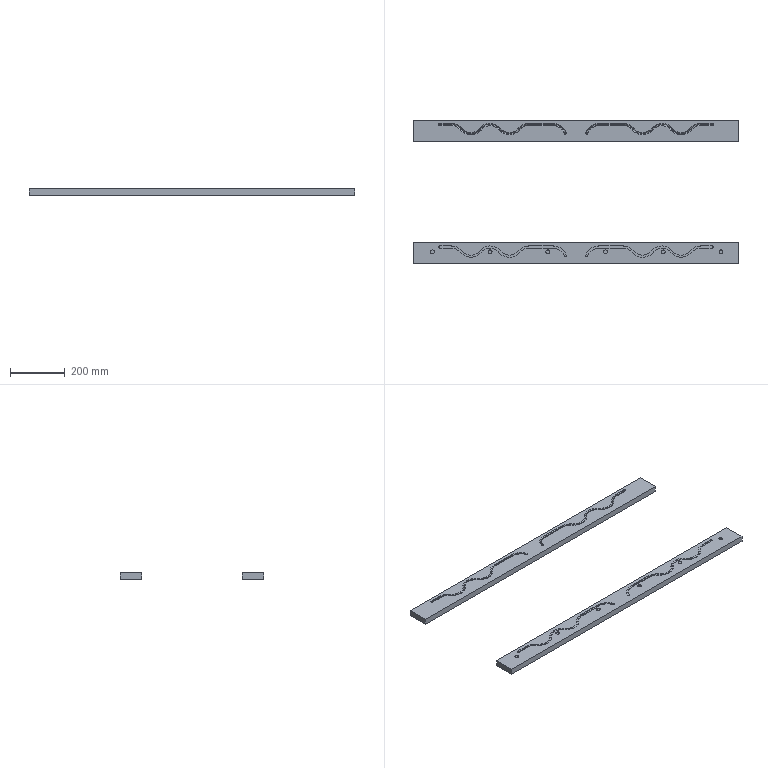NC program | NX | posted with a generic post | part box 1185 x 523.484 x 22 mm
Lines 1046 to 2009 of 261559:
(定轴曲面加工 , TOOL : D3平底刀)
N2072 T15 M6
N2074 /M1
N2076 G54
N2078 G17 G0 G90 X22.96 Y24.701 S3000 M3
N2080 G43 Z50. H15
N2082 Z1.5
N2084 G94 G1 X23.024 Y24.738 Z1.036 F2450.
N2086 X23.208 Y24.845 Z0.618
N2088 X23.495 Y25.012 Z0.286
N2090 X23.856 Y25.223 Z0.073
N2092 X24.257 Y25.456 Z0.
N2094 X24.643 Y25.681 F3500.
N2096 X25.42 Y26.134
N2098 X25.799 Y26.355
N2100 X25.809 Y26.359
N2102 X26.024 Y26.417
N2104 X26.049 Y26.42
N2106 X26.06 Y26.394
N2108 X26.039 Y26.379
N2110 X25.471 Y26.048
N2112 X24.693 Y25.595
N2114 X24. Y25.191
N2116 X23.995 Y25.187
N2118 X23.982 Y25.174
N2120 X23.826 Y24.987
N2122 X23.822 Y24.983
N2124 X23.826 Y24.98
N2126 X23.83 Y24.975
N2128 X23.834 Y24.979
N2130 X23.966 Y25.055
N2132 X24.743 Y25.508
N2134 X25.521 Y25.961
N2136 X26.299 Y26.414
N2138 X26.446 Y26.5
N2140 X26.464 Y26.506
N2142 X26.537 Y26.515
N2144 X26.573 Y26.512
N2146 X26.585 Y26.474
N2148 X26.558 Y26.45
N2150 X26.349 Y26.328
N2152 X25.571 Y25.875
N2154 X24.794 Y25.422
N2156 X24.016 Y24.969
N2158 X23.673 Y24.769
N2160 X23.666 Y24.762
N2162 X23.65 Y24.743
N2164 X23.571 Y24.621
N2166 X23.563 Y24.612
N2168 X23.572 Y24.605
N2170 X23.579 Y24.596
N2172 X23.587 Y24.603
N2174 X24.066 Y24.882
N2176 X24.844 Y25.335
N2178 X25.622 Y25.789
N2180 X26.399 Y26.242
N2182 X26.906 Y26.537
N2184 X26.929 Y26.544
N2186 X26.975 Y26.546
N2188 X27.013 Y26.54
N2190 X27.025 Y26.5
N2192 X26.997 Y26.474
N2194 X26.45 Y26.155
N2196 X25.672 Y25.702
N2198 X24.894 Y25.249
N2200 X24.117 Y24.796
N2202 X23.459 Y24.413
N2204 X23.45 Y24.404
N2206 X23.433 Y24.38
N2208 X23.391 Y24.298
N2210 X23.38 Y24.285
N2212 X23.395 Y24.276
N2214 X23.405 Y24.261
N2216 X23.418 Y24.273
N2218 X24.167 Y24.71
N2220 X24.945 Y25.163
N2222 X25.722 Y25.616
N2224 X26.5 Y26.069
N2226 X27.278 Y26.522
N2228 X27.328 Y26.551
N2230 X27.353 Y26.558
N2232 X27.395
N2234 X27.432 Y26.551
N2236 X27.443 Y26.512
N2238 X27.415 Y26.486
N2240 X27.328 Y26.436
N2242 X26.55 Y25.983
N2244 X25.773 Y25.529
N2246 X24.995 Y25.076
N2248 X24.217 Y24.623
N2250 X23.44 Y24.17
N2252 X23.306 Y24.092
N2254 X23.296 Y24.081
N2256 X23.279 Y24.053
N2258 X23.251 Y23.985
N2260 X23.241 Y23.971
N2262 X23.256 Y23.964
N2264 X23.267 Y23.949
N2266 X23.28 Y23.961
N2268 X23.49 Y24.084
N2270 X24.268 Y24.537
N2272 X25.045 Y24.99
N2274 X25.823 Y25.443
N2276 X26.601 Y25.896
N2278 X27.378 Y26.349
N2280 X27.73 Y26.554
N2282 X27.755 Y26.561
N2284 X27.797 Y26.562
N2286 X27.835 Y26.554
N2288 X27.846 Y26.515
N2290 X27.817 Y26.489
N2292 X27.429 Y26.263
N2294 X26.651 Y25.81
N2296 X25.873 Y25.357
N2298 X25.096 Y24.904
N2300 X24.318 Y24.45
N2302 X23.54 Y23.997
N2304 X23.194 Y23.796
N2306 X23.184 Y23.783
N2308 X23.166 Y23.75
N2310 X23.148 Y23.693
N2312 X23.139 Y23.679
N2314 X23.154 Y23.673
N2316 X23.155 Y23.672
N2318 X23.165 Y23.658
N2320 X23.178 Y23.67
N2322 X23.591 Y23.911
N2324 X24.368 Y24.364
N2326 X25.146 Y24.817
N2328 X25.924 Y25.27
N2330 X26.701 Y25.723
N2332 X27.479 Y26.177
N2334 X28.133 Y26.558
N2336 X28.157 Y26.564
N2338 X28.2 Y26.565
N2340 X28.237 Y26.557
N2342 X28.248 Y26.518
N2344 X28.22 Y26.492
N2346 X27.529 Y26.09
N2348 X26.752 Y25.637
N2350 X25.974 Y25.184
N2352 X25.196 Y24.731
N2354 X24.419 Y24.278
N2356 X23.641 Y23.825
N2358 X23.112 Y23.516
N2360 X23.101 Y23.502
N2362 X23.084 Y23.466
N2364 X23.076 Y23.433
N2366 X23.067 Y23.415
N2368 X23.086 Y23.406
N2370 X23.087
N2372 X23.101 Y23.39
N2374 X23.118 Y23.404
N2376 X23.691 Y23.738
N2378 X24.469 Y24.191
N2380 X25.247 Y24.644
N2382 X26.024 Y25.098
N2384 X26.802 Y25.551
N2386 X27.58 Y26.004
N2388 X28.357 Y26.457
N2390 X28.535 Y26.561
N2392 X28.56 Y26.567
N2394 X28.602 Y26.568
N2396 X28.639 Y26.56
N2398 X28.65 Y26.521
N2400 X28.622 Y26.495
N2402 X28.408 Y26.37
N2404 X27.63 Y25.917
N2406 X26.852 Y25.464
N2408 X26.075 Y25.011 Z-0.001
N2410 X25.297 Y24.558 Z-0.002
N2412 X24.519 Y24.105 Z0.
N2414 X23.742 Y23.652
N2416 X23.054 Y23.251
N2418 X23.043 Y23.235
N2420 X23.023 Y23.22
N2422 X23.027 Y23.195
N2424 X23.022 Y23.171
N2426 X23.015 Y23.151
N2428 X23.034 Y23.143
N2430 X23.049 Y23.128
N2432 X23.064 Y23.141
N2434 X23.792 Y23.565
N2436 X24.57 Y24.019
N2438 X25.347 Y24.472 Z-0.011
N2440 X26.125 Y24.925
N2442 X26.903 Y25.378 Z0.
N2444 X27.68 Y25.831
N2446 X28.458 Y26.284
N2448 X28.934 Y26.561
N2450 X28.959 Y26.568
N2452 X29.
N2454 X29.038 Y26.561
N2456 X29.048 Y26.521
N2458 X29.02 Y26.496
N2460 X28.508 Y26.198
N2462 X27.731 Y25.745
N2464 X26.953 Y25.292
N2466 X26.175 Y24.838 Z-0.02
N2468 X25.398 Y24.385 Z-0.021
N2470 X24.62 Y23.932 Z0.
N2472 X23.842 Y23.479
N2474 X23.065 Y23.026
N2476 X23.016 Y22.998
N2478 X23.005 Y22.98
N2480 X22.985 Y22.963
N2482 X22.989 Y22.937
N2484 Y22.932
N2486 X22.983 Y22.909
N2488 X23.004 Y22.899
N2490 X23.006 Y22.898
N2492 X23.024 Y22.882
N2494 X23.042 Y22.897
N2496 X23.115 Y22.94
N2498 X23.893 Y23.393
N2500 X24.67 Y23.846
N2502 X25.448 Y24.299 Z-0.031
N2504 X26.226 Y24.752 Z-0.03
N2506 X27.003 Y25.205 Z0.
N2508 X27.781 Y25.658
N2510 X28.559 Y26.111
N2512 X29.331 Y26.562
N2514 X29.356 Y26.568
N2516 X29.398
N2518 X29.435 Y26.561
N2520 X29.446 Y26.521
N2522 X29.417 Y26.496
N2524 X29.386 Y26.478
N2526 X28.609 Y26.025
N2528 X27.831 Y25.572
N2530 X27.054 Y25.119 Z-0.005
N2532 X26.276 Y24.666 Z-0.04
N2534 X25.498 Y24.213
N2536 X24.721 Y23.759 Z-0.008
N2538 X23.943 Y23.306 Z0.
N2540 X23.166 Y22.853
N2542 X23.015 Y22.765
N2544 X22.99 Y22.759
N2546 X22.983 Y22.735
N2548 X22.982 Y22.733
N2550 X22.963 Y22.716
N2552 X22.969 Y22.691
N2554 Y22.688
N2556 X22.964 Y22.665
N2558 X22.986 Y22.656
N2560 X23.005 Y22.641
N2562 X23.025 Y22.656
N2564 X23.216 Y22.767
N2566 X23.993 Y23.22
N2568 X24.771 Y23.673 Z-0.017
N2570 X25.549 Y24.126 Z-0.068
N2572 X26.326 Y24.579 Z-0.066
N2574 X27.104 Y25.032 Z-0.011
N2576 X27.882 Y25.485 Z0.
N2578 X28.659 Y25.939
N2580 X29.437 Y26.392
N2582 X29.728 Y26.562
N2584 X29.754 Y26.568
N2586 X29.795
N2588 X29.833 Y26.561
N2590 X29.843 Y26.521
N2592 X29.815 Y26.496
N2594 X29.487 Y26.305
N2596 X28.71 Y25.852
N2598 X27.932 Y25.399
N2600 X27.154 Y24.946 Z-0.016
N2602 X26.377 Y24.493 Z-0.096
N2604 X25.599 Y24.04 Z-0.097
N2606 X24.821 Y23.587 Z-0.025
N2608 X24.044 Y23.134 Z0.
N2610 X23.266 Y22.68
N2612 X23.009 Y22.531
N2614 X22.984 Y22.524
N2616 X22.977 Y22.498
N2618 X22.974 Y22.493
N2620 X22.957 Y22.477
N2622 X22.964 Y22.456
N2624 Y22.452
N2626 X22.96 Y22.43
N2628 X22.982 Y22.422
N2630 X23.002 Y22.407
N2632 X23.021 Y22.422
N2634 X23.317 Y22.594
N2636 X24.094 Y23.047
N2638 X24.872 Y23.5 Z-0.033
N2640 X25.645 Y23.951 Z-0.127
N2642 X25.649 Y23.953
N2644 X25.654 Y23.956
N2646 X26.422 Y24.404 Z-0.126
N2648 X26.427 Y24.407
N2650 X26.432 Y24.409 Z-0.125
N2652 X27.205 Y24.86 Z-0.028
N2654 X27.982 Y25.313 Z0.
N2656 X28.76 Y25.766
N2658 X29.537 Y26.219
N2660 X30.126 Y26.562
N2662 X30.151 Y26.569
N2664 X30.193
N2666 X30.23 Y26.561
N2668 X30.241 Y26.522
N2670 X30.212 Y26.496
N2672 X29.588 Y26.133
N2674 X28.81 Y25.679
N2676 X28.033 Y25.226
N2678 X27.255 Y24.773 Z-0.042
N2680 X26.477 Y24.32 Z-0.155
N2682 X26.092 Y24.096 Z-0.176
N2684 X26.089 Y24.094
N2686 X26.085 Y24.091
N2688 X25.7 Y23.867 Z-0.157
N2690 X24.922 Y23.414 Z-0.042
N2692 X24.144 Y22.961 Z0.
N2694 X23.367 Y22.508
N2696 X23.018 Y22.304
N2698 X22.991 Y22.296
N2700 X22.984 Y22.269
N2702 X22.978 Y22.259
N2704 X22.972 Y22.23
N2706 Y22.228
N2708 X22.968 Y22.209
N2710 X22.987 Y22.205
N2712 X22.989 Y22.204
N2714 X23.018 Y22.187
N2716 X23.046 Y22.205
N2718 X23.417 Y22.421
N2720 X24.195 Y22.874
N2722 X24.972 Y23.328 Z-0.065
N2724 X25.746 Y23.778 Z-0.201
N2726 X25.75 Y23.781 Z-0.202
N2728 X25.754 Y23.783
N2730 X26.133 Y24.004 Z-0.229
N2732 X26.139 Y24.007 Z-0.23
N2734 X26.145 Y24.011 Z-0.229
N2736 X26.528 Y24.234 Z-0.197
N2738 X27.305 Y24.687 Z-0.062
N2740 X28.083 Y25.14 Z-0.004
N2742 X28.861 Y25.593 Z0.
N2744 X29.638 Y26.046
N2746 X30.416 Y26.499
N2748 X30.523 Y26.562
N2750 X30.548 Y26.569
N2752 X30.59
N2754 X30.627 Y26.561
N2756 X30.638 Y26.522
N2758 X30.61 Y26.497
N2760 X30.466 Y26.413
N2762 X29.688 Y25.96
N2764 X28.911 Y25.507
N2766 X28.133 Y25.054 Z-0.009
N2768 X27.356 Y24.6 Z-0.085
N2770 X26.582 Y24.15 Z-0.248
N2772 X26.578 Y24.147
N2774 X26.574 Y24.145 Z-0.249
N2776 X26.195 Y23.924 Z-0.283
N2778 X26.189 Y23.921
N2780 X26.183 Y23.917
N2782 X25.805 Y23.697 Z-0.254
N2784 X25.8 Y23.694
N2786 X25.795 Y23.691 Z-0.253
N2788 X25.023 Y23.241 Z-0.088
N2790 X24.634 Y23.015 Z-0.026
N2792 X24.245 Y22.788 Z0.
N2794 X23.468 Y22.335
N2796 X23.038 Y22.085
N2798 X23.01 Y22.075
N2800 X23.003 Y22.047
N2802 X22.997 Y22.035
N2804 X22.992 Y22.008
N2806 Y22.007
N2808 X22.989 Y21.988
N2810 X23.008 Y21.985
N2812 X23.01 Y21.984
N2814 X23.039 Y21.967
N2816 X23.066 Y21.985
N2818 X23.518 Y22.249
N2820 X24.295 Y22.702
N2822 X24.684 Y22.928 Z-0.033
N2824 X25.073 Y23.155 Z-0.112
N2826 X25.845 Y23.604 Z-0.303
N2828 X25.851 Y23.608 Z-0.305
N2830 X25.857 Y23.611
N2832 X26.233 Y23.831 Z-0.336
N2834 X26.24 Y23.834 Z-0.337
N2836 X26.246 Y23.838 Z-0.336
N2838 X26.623 Y24.058 Z-0.301
N2840 X26.628 Y24.061 Z-0.3
N2842 X26.634 Y24.064 Z-0.299
N2844 X27.017 Y24.288 Z-0.201
N2846 X27.406 Y24.514 Z-0.114
N2848 X28.184 Y24.967 Z-0.015
N2850 X28.961 Y25.42 Z0.
N2852 X29.739 Y25.873
N2854 X30.516 Y26.327
N2856 X30.921 Y26.562
N2858 X30.946 Y26.569
N2860 X30.987
N2862 X31.025 Y26.562
N2864 X31.036 Y26.522
N2866 X31.007 Y26.497
N2868 X30.567 Y26.24
N2870 X29.789 Y25.787
N2872 X29.012 Y25.334
N2874 X28.234 Y24.881 Z-0.024
N2876 X27.456 Y24.428 Z-0.143
N2878 X27.067 Y24.201 Z-0.244
N2880 X26.873 Y24.088 Z-0.302
N2882 X26.683 Y23.977 Z-0.35
N2884 X26.679 Y23.975 Z-0.351
N2886 X26.674 Y23.972 Z-0.352
N2888 X26.299 Y23.753 Z-0.4
N2890 X26.29 Y23.748 Z-0.401
N2892 X26.281 Y23.743 Z-0.4
N2894 X25.907 Y23.525 Z-0.356
N2896 X25.901 Y23.522
N2898 X25.895 Y23.518 Z-0.354
N2900 X25.123 Y23.068 Z-0.135
N2902 X24.735 Y22.842 Z-0.039
N2904 X24.346 Y22.615 Z-0.003
N2906 X23.568 Y22.162 Z0.
N2908 X23.069 Y21.872
N2910 X23.041 Y21.861
N2912 X23.033 Y21.832
N2914 X23.025 Y21.815
N2916 X23.023 Y21.796
N2918 Y21.795
N2920 X23.019 Y21.78
N2922 X23.035
N2924 X23.038 Y21.778
N2926 X23.062 Y21.761
N2928 X23.091 Y21.762
N2930 X23.113 Y21.781
N2932 X23.619 Y22.076
N2934 X24.396 Y22.529 Z-0.008
N2936 X24.785 Y22.755 Z-0.053
N2938 X25.174 Y22.982 Z-0.156
N2940 X25.944 Y23.431 Z-0.424
N2942 X25.951 Y23.435 Z-0.426
N2944 X25.959 Y23.439 Z-0.427
N2946 X26.329 Y23.655 Z-0.482
N2948 X26.34 Y23.662 Z-0.483
N2950 X26.352 Y23.668 Z-0.482
N2952 X26.723 Y23.884 Z-0.421
N2954 X26.729 Y23.888 Z-0.42
N2956 X26.735 Y23.892 Z-0.418
N2958 X26.923 Y24.002 Z-0.352
N2960 X27.118 Y24.115 Z-0.287
N2962 X27.507 Y24.341 Z-0.175
N2964 X28.284 Y24.794 Z-0.038
N2966 X29.062 Y25.248 Z0.
N2968 X29.839 Y25.701
N2970 X30.617 Y26.154
N2972 X31.318 Y26.562
N2974 X31.343 Y26.569
N2976 X31.385
N2978 X31.422 Y26.562
N2980 X31.433 Y26.522
N2982 X31.404 Y26.497
N2984 X30.667 Y26.067
N2986 X29.89 Y25.614
N2988 X29.112 Y25.161 Z-0.002
N2990 X28.335 Y24.708 Z-0.057
N2992 X27.557 Y24.255 Z-0.218
N2994 X26.785 Y23.805 Z-0.494
N2996 X26.779 Y23.802 Z-0.496
N2998 X26.773 Y23.798 Z-0.497
N3000 X26.403 Y23.583 Z-0.563
N3002 X26.391 Y23.575 Z-0.565
N3004 X26.378 Y23.568 Z-0.564
N3006 X26.011 Y23.354 Z-0.506
N3008 X26.002 Y23.349 Z-0.504
N3010 X25.993 Y23.344 Z-0.501
N3012 X25.224 Y22.896 Z-0.185
N3014 X24.835 Y22.669 Z-0.07
N3016 X24.446 Y22.443 Z-0.013
N3018 X23.669 Y21.989 Z0.
N3020 X23.111 Y21.665
N3022 X23.082 Y21.653
N3024 X23.074 Y21.623
N3026 X23.067 Y21.605
N3028 X23.065 Y21.586
N3030 X23.062 Y21.571
N3032 X23.076 Y21.572
N3034 X23.077 Y21.571
N3036 X23.103 Y21.554
N3038 X23.134 Y21.556
N3040 X23.158 Y21.576
N3042 X23.719 Y21.903
N3044 X24.497 Y22.356 Z-0.018
N3046 X24.886 Y22.583 Z-0.087
N3048 X25.274 Y22.809 Z-0.221
N3050 X26.043 Y23.257 Z-0.578
N3052 X26.052 Y23.262 Z-0.581
N3054 X26.062 Y23.268 Z-0.584
N3056 X26.427 Y23.481 Z-0.648
N3058 X26.441 Y23.489 Z-0.649
N3060 X26.455 Y23.497 Z-0.647
N3062 X26.823 Y23.711 Z-0.574
N3064 X26.83 Y23.715 Z-0.572
N3066 X26.836 Y23.719 Z-0.57
N3068 X27.607 Y24.169 Z-0.26
N3070 X28.385 Y24.622 Z-0.078
N3072 X29.163 Y25.075 Z-0.008
N3074 X29.94 Y25.528 Z0.
N3076 X30.718 Y25.981
N3078 X31.495 Y26.434
N3080 X31.716 Y26.562
N3082 X31.741 Y26.569
N3084 X31.782
N3086 X31.82 Y26.562
N3088 X31.83 Y26.522
N3090 X31.802 Y26.497
N3092 X31.546 Y26.348
N3094 X30.768 Y25.895
N3096 X29.99 Y25.442
N3098 X29.213 Y24.988 Z-0.013
N3100 X28.435 Y24.535 Z-0.107
N3102 X27.658 Y24.082 Z-0.306
N3104 X27.269 Y23.856 Z-0.47
N3106 X27.074 Y23.742 Z-0.563
N3108 X26.88 Y23.629 Z-0.651
N3110 X26.695 Y23.521 Z-0.735
N3112 X26.685 Y23.516 Z-0.738
N3114 X26.676 Y23.51 Z-0.741
N3116 X26.502 Y23.409 Z-0.77
N3118 X26.491 Y23.403 Z-0.771
N3120 X26.48 Y23.396 Z-0.77
N3122 X26.307 Y23.295 Z-0.747
N3124 X26.297 Y23.289 Z-0.745
N3126 X26.287 Y23.284 Z-0.742
N3128 X26.102 Y23.176 Z-0.664
N3130 X25.325 Y22.723 Z-0.254
N3132 X24.936 Y22.496 Z-0.103
N3134 X24.547 Y22.27 Z-0.022
N3136 X23.77 Y21.817 Z0.
N3138 X23.137 Y21.448
N3140 X23.118 Y21.4
N3142 X23.117 Y21.382
N3144 X23.114 Y21.367
N3146 X23.129 Y21.368
N3148 X23.13
N3150 X23.155 Y21.352
N3152 X23.185 Y21.354
N3154 X23.208 Y21.374
N3156 X23.82 Y21.73
N3158 X24.597 Y22.183 Z-0.026
N3160 X24.986 Y22.41 Z-0.117
N3162 X25.375 Y22.637 Z-0.287
N3164 X25.764 Y22.863 Z-0.523
N3166 X26.148 Y23.087 Z-0.773
N3168 X26.153 Y23.09 Z-0.776
N3170 X26.158 Y23.093 Z-0.779
N3172 X26.337 Y23.197 Z-0.86
N3174 X26.347 Y23.203 Z-0.864
N3176 X26.358 Y23.209 Z-0.866
N3178 X26.529 Y23.309 Z-0.892
N3180 X26.541 Y23.316
N3182 X26.554 Y23.323 Z-0.891
N3184 X26.725 Y23.423 Z-0.859
N3186 X26.736 Y23.429 Z-0.856
N3188 X26.746 Y23.435 Z-0.852
N3190 X26.93 Y23.543 Z-0.76
N3192 X27.319 Y23.769 Z-0.541
N3194 X27.708 Y23.996 Z-0.359
N3196 X28.486 Y24.449 Z-0.136
N3198 X29.263 Y24.902 Z-0.02
N3200 X30.041 Y25.355 Z0.
N3202 X30.818 Y25.808
N3204 X31.596 Y26.261
N3206 X32.113 Y26.563
N3208 X32.138 Y26.569
N3210 X32.18
N3212 X32.217 Y26.562
N3214 X32.228 Y26.522
N3216 X32.199 Y26.497
N3218 X31.646 Y26.175
N3220 X30.869 Y25.722
N3222 X30.091 Y25.269
N3224 X29.314 Y24.816 Z-0.035
N3226 X28.536 Y24.363 Z-0.166
N3228 X28.147 Y24.136 Z-0.277
N3230 X27.758 Y23.909 Z-0.426
N3232 X27.369 Y23.683 Z-0.612
N3234 X26.981 Y23.456 Z-0.869
N3236 X26.793 Y23.347 Z-0.971
N3238 X26.786 Y23.343 Z-0.975
N3240 X26.779 Y23.339 Z-0.977
N3242 X26.612 Y23.242 Z-1.03
N3244 X26.592 Y23.23 Z-1.033
N3246 X26.571 Y23.218 Z-1.031
N3248 X26.407 Y23.122 Z-0.99
N3250 X26.398 Y23.117 Z-0.988
N3252 X26.389 Y23.111 Z-0.984
N3254 X26.21 Y23.007 Z-0.889
N3256 X26.203 Y23.003 Z-0.885
N3258 X26.197 Y23. Z-0.881
N3260 X25.814 Y22.777 Z-0.581
N3262 X25.425 Y22.55 Z-0.316
N3264 X25.037 Y22.324 Z-0.131
N3266 X24.648 Y22.097 Z-0.03
N3268 X24.259 Y21.87 Z0.
N3270 X23.87 Y21.644
N3272 X23.225 Y21.268
N3274 X23.196 Y21.256
N3276 X23.189 Y21.226
N3278 X23.179 Y21.199
N3280 Y21.188
N3282 X23.178 Y21.178
N3284 X23.187 Y21.18
N3286 X23.195 Y21.177
N3288 X23.223 Y21.161
N3290 X23.255 Y21.164
N3292 X23.28 Y21.184
N3294 X23.92 Y21.558
N3296 X24.309 Y21.784
N3298 X24.698 Y22.011 Z-0.033
N3300 X25.087 Y22.237 Z-0.143
N3302 X25.476 Y22.464 Z-0.343
N3304 X25.865 Y22.69 Z-0.635
N3306 X26.253 Y22.917 Z-1.
N3308 X26.434 Y23.022 Z-1.156
N3310 X26.449 Y23.031 Z-1.166
N3312 X26.465 Y23.04 Z-1.173
N3314 X26.619 Y23.13 Z-1.217
N3316 X26.642 Y23.143 Z-1.219
N3318 X26.665 Y23.157 Z-1.215
N3320 X26.822 Y23.248 Z-1.158
N3322 X26.836 Y23.256 Z-1.151
N3324 X26.849 Y23.264 Z-1.141
N3326 X26.934 Y23.313 Z-1.064
N3328 X27.031 Y23.37 Z-0.979
N3330 X27.42 Y23.597 Z-0.701
N3332 X27.809 Y23.823 Z-0.496
N3334 X28.197 Y24.05 Z-0.326
N3336 X28.586 Y24.276 Z-0.207
N3338 X29.364 Y24.729 Z-0.052
N3340 X30.141 Y25.182 Z-0.001
N3342 X30.919 Y25.635 Z0.
N3344 X31.697 Y26.089
N3346 X32.474 Y26.542
N3348 X32.51 Y26.563
N3350 X32.535 Y26.569
N3352 X32.567
N3354 X32.577
N3356 X32.614 Y26.562
N3358 X32.625 Y26.522
N3360 X32.597 Y26.497
N3362 X32.525 Y26.455
N3364 X31.747 Y26.002
N3366 X30.969 Y25.549
N3368 X30.192 Y25.096 Z-0.006
N3370 X29.414 Y24.643 Z-0.072
N3372 X28.637 Y24.19 Z-0.25
N3374 X28.248 Y23.963 Z-0.381
N3376 X27.859 Y23.737 Z-0.567
N3378 X27.47 Y23.51 Z-0.806
N3380 X27.081 Y23.284 Z-1.122
N3382 X26.895 Y23.175 Z-1.32
N3384 X26.887 Y23.17 Z-1.328
N3386 X26.878 Y23.165 Z-1.334
N3388 X26.72 Y23.073 Z-1.433
N3390 X26.692 Y23.057 Z-1.444
N3392 X26.661 Y23.039 Z-1.443
N3394 X26.613 Y23.011 Z-1.431
N3396 X26.596 Y23.001 Z-1.425
N3398 X26.581 Y22.992 Z-1.415
N3400 X26.498 Y22.944 Z-1.347
N3402 X26.307 Y22.832 Z-1.161
N3404 X26.304 Y22.831 Z-1.158
N3406 X26.301 Y22.829 Z-1.155
N3408 X25.915 Y22.604 Z-0.707
N3410 X25.526 Y22.377 Z-0.368
N3412 X25.137 Y22.151 Z-0.154
N3414 X24.748 Y21.924 Z-0.036
N3416 X24.36 Y21.698 Z0.
N3418 X23.971 Y21.471
N3420 X23.297 Y21.079
N3422 X23.268 Y21.066
N3424 X23.261 Y21.035
N3426 X23.252 Y21.007
N3428 Y20.996
N3430 X23.251 Y20.987
N3432 X23.26 Y20.989
N3434 X23.268 Y20.986
N3436 X23.312 Y20.971
N3438 X23.351 Y20.994
N3440 X24.021 Y21.385
N3442 X24.41 Y21.611
N3444 X24.799 Y21.838 Z-0.038
N3446 X25.188 Y22.064 Z-0.164
N3448 X25.576 Y22.291 Z-0.399
N3450 X25.771 Y22.404 Z-0.568
N3452 X25.965 Y22.518 Z-0.773
N3454 X26.16 Y22.631 Z-1.008
N3456 X26.354 Y22.744 Z-1.308
N3458 X26.542 Y22.854 Z-1.639
N3460 X26.549 Y22.858 Z-1.649
N3462 X26.557 Y22.862 Z-1.658
N3464 X26.634 Y22.907 Z-1.739
N3466 X26.646 Y22.914 Z-1.75
N3468 X26.66 Y22.923 Z-1.758
N3470 X26.705 Y22.948 Z-1.778
N3472 X26.742 Y22.97 Z-1.785
N3474 X26.779 Y22.991 Z-1.773
N3476 X26.826 Y23.019 Z-1.742
N3478 X26.839 Y23.027 Z-1.731
N3480 X26.85 Y23.033 Z-1.719
N3482 X26.934 Y23.082 Z-1.603
N3484 X26.937 Y23.084 Z-1.599
N3486 X26.94 Y23.085 Z-1.595
N3488 X27.034 Y23.141 Z-1.436
N3490 X27.132 Y23.197 Z-1.297
N3492 X27.326 Y23.31 Z-1.075
N3494 X27.52 Y23.424 Z-0.912
N3496 X27.909 Y23.65 Z-0.639
N3498 X28.687 Y24.103 Z-0.293
N3500 X29.465 Y24.557 Z-0.1
N3502 X30.242 Y25.01 Z-0.012
N3504 X31.02 Y25.463 Z0.
N3506 X31.797 Y25.916
N3508 X32.575 Y26.369
N3510 X32.907 Y26.562
N3512 X32.932 Y26.569
N3514 X32.973
N3516 X33.011 Y26.562
N3518 X33.021 Y26.522
N3520 X32.993 Y26.497
N3522 X32.625 Y26.283
N3524 X31.848 Y25.829
N3526 X31.07 Y25.376
N3528 X30.292 Y24.923 Z-0.018
N3530 X29.515 Y24.47 Z-0.129
N3532 X28.737 Y24.017 Z-0.346
N3534 X28.348 Y23.79 Z-0.523
N3536 X27.96 Y23.564 Z-0.741
N3538 X27.571 Y23.337 Z-1.031
N3540 X27.376 Y23.224 Z-1.242
N3542 X27.182 Y23.111 Z-1.524
N3544 X27.045 Y23.031 Z-1.847
N3546 X27.046 Y23.029 Z-1.86
N3548 X27.083 Y23.021 Z-1.916
N3550 X27.15 Z-1.909
N3552 X27.176 Y23.023 Z-1.89
N3554 X27.178
N3556 X27.213 Y23.025 Z-1.88
N3558 X27.241 Y23.03 Z-1.857
N3560 X27.242 Z-1.854
N3562 X27.338 Y23.086 Z-1.598
N3564 X27.434 Y23.142 Z-1.433
N3566 X27.626 Y23.254 Z-1.182
N3568 X27.818 Y23.366 Z-0.986
N3570 X28.01 Y23.478 Z-0.846
N3572 X28.399 Y23.704 Z-0.594
N3574 X28.788 Y23.931 Z-0.408
N3576 X29.565 Y24.384 Z-0.158
N3578 X30.343 Y24.837 Z-0.031
N3580 X31.12 Y25.29 Z0.
N3582 X31.898 Y25.743
N3584 X32.676 Y26.196
N3586 X33.304 Y26.562
N3588 X33.329 Y26.569
N3590 X33.371
N3592 X33.408 Y26.562
N3594 X33.419 Y26.522
N3596 X33.39 Y26.497
N3598 X32.726 Y26.11
N3600 X31.948 Y25.657
N3602 X31.171 Y25.204
N3604 X30.393 Y24.75 Z-0.047
N3606 X29.616 Y24.297 Z-0.197
N3608 X29.227 Y24.071 Z-0.313
N3610 X28.838 Y23.844 Z-0.479
N3612 X28.449 Y23.618 Z-0.675
N3614 X28.06 Y23.391 Z-0.951
N3616 X27.76 Y23.216 Z-1.258
N3618 X27.61 Y23.129 Z-1.47
N3620 X27.46 Y23.042 Z-1.796
N3622 X27.462 Y23.036 Z-1.822
N3624 X27.484 Y23.027 Z-1.87
N3626 X27.535 Y23.023 Z-1.89
N3628 X27.572
N3630 X27.609 Y23.025 Z-1.881
N3632 X27.638 Y23.03 Z-1.857
N3634 X27.639 Z-1.854
N3636 X27.757 Y23.099 Z-1.56
N3638 X27.875 Y23.167 Z-1.359
N3640 X28.111 Y23.305 Z-1.084
N3642 X28.499 Y23.531 Z-0.781
N3644 X28.888 Y23.758 Z-0.55
N3646 X29.277 Y23.984 Z-0.366
N3648 X29.666 Y24.211 Z-0.24
N3650 X30.443 Y24.664 Z-0.067
N3652 X31.221 Y25.117 Z-0.005
N3654 X31.999 Y25.57 Z0.
N3656 X32.776 Y26.023
N3658 X33.554 Y26.477
N3660 X33.702 Y26.563
N3662 X33.727 Y26.569
N3664 X33.768
N3666 X33.806 Y26.562
N3668 X33.816 Y26.522
N3670 X33.788 Y26.497
N3672 X33.604 Y26.39
N3674 X32.827 Y25.937
N3676 X32.049 Y25.484
N3678 X31.271 Y25.031 Z-0.011
N3680 X30.494 Y24.578 Z-0.092
N3682 X29.716 Y24.125 Z-0.282
N3684 X28.939 Y23.672 Z-0.621
N3686 X28.55 Y23.445 Z-0.886
N3688 X28.355 Y23.332 Z-1.04
N3690 X28.161 Y23.218 Z-1.254
N3692 X28.009 Y23.13 Z-1.467
N3694 X27.858 Y23.042 Z-1.796
N3696 X27.859 Y23.037 Z-1.822
N3698 X27.882 Y23.027 Z-1.87
N3700 X27.932 Y23.023 Z-1.889
N3702 X27.969
N3704 X28.006 Y23.025 Z-1.881
N3706 X28.035 Y23.03 Z-1.856
N3708 X28.036 Z-1.854
N3710 X28.124 Y23.081 Z-1.612
N3712 X28.211 Y23.132 Z-1.461
N3714 X28.406 Y23.245 Z-1.199
N3716 X28.6 Y23.359 Z-0.997
N3718 X28.989 Y23.585 Z-0.715
N3720 X29.378 Y23.812 Z-0.506
N3722 X29.767 Y24.038 Z-0.333
N3724 X30.544 Y24.491 Z-0.122
N3726 X31.322 Y24.944 Z-0.016
N3728 X32.099 Y25.398 Z0.
N3730 X32.877 Y25.851
N3732 X33.655 Y26.304
N3734 X34.099 Y26.563
N3736 X34.124 Y26.57
N3738 X34.166
N3740 X34.204 Y26.562
N3742 X34.214 Y26.523
N3744 X34.186 Y26.498
N3746 X33.705 Y26.217
N3748 X32.927 Y25.764
N3750 X32.15 Y25.311
N3752 X31.372 Y24.858 Z-0.028
N3754 X30.594 Y24.405 Z-0.151
N3756 X29.817 Y23.952 Z-0.391
N3758 X29.428 Y23.725 Z-0.577
N3760 X29.039 Y23.499 Z-0.82
N3762 X28.843 Y23.384 Z-0.96
N3764 X28.647 Y23.27 Z-1.149
N3766 X28.451 Y23.156 Z-1.391
N3768 X28.353 Y23.099 Z-1.559
N3770 X28.255 Y23.042 Z-1.796
N3772 X28.256 Y23.037 Z-1.821
N3774 X28.279 Y23.027 Z-1.87
N3776 X28.329 Y23.023 Z-1.889
N3778 X28.367
N3780 X28.403 Y23.025 Z-1.88
N3782 X28.432 Y23.03 Z-1.856
N3784 X28.434 Z-1.854
N3786 X28.515 Y23.078 Z-1.621
N3788 X28.597 Y23.125 Z-1.48
N3790 X28.761 Y23.221 Z-1.248
N3792 X29.09 Y23.412 Z-0.926
N3794 X29.478 Y23.639 Z-0.65
N3796 X29.867 Y23.865 Z-0.462
N3798 X30.256 Y24.092 Z-0.3
N3800 X30.645 Y24.319 Z-0.186
N3802 X31.422 Y24.772 Z-0.042
N3804 X32.2 Y25.225 Z0.
N3806 X32.978 Y25.678
N3808 X33.755 Y26.131
N3810 X34.497 Y26.563
N3812 X34.522 Y26.57
N3814 X34.526
N3816 X34.564
N3818 X34.601 Y26.563
N3820 X34.612 Y26.523
N3822 X34.584 Y26.498
N3824 X33.806 Y26.045
N3826 X33.028 Y25.592
N3828 X32.25 Y25.138 Z-0.004
N3830 X31.473 Y24.685 Z-0.062
N3832 X30.695 Y24.232 Z-0.229
N3834 X30.306 Y24.006 Z-0.353
N3836 X29.917 Y23.779 Z-0.533
N3838 X29.529 Y23.553 Z-0.755
N3840 X29.14 Y23.326 Z-1.05
N3842 X28.896 Y23.184 Z-1.324
N3844 X28.774 Y23.113 Z-1.518
N3846 X28.652 Y23.042 Z-1.795
N3848 X28.653 Y23.037 Z-1.821
N3850 X28.676 Y23.027 Z-1.869
N3852 X28.726 Y23.023 Z-1.889
N3854 X28.764
N3856 X28.801 Y23.025 Z-1.88
N3858 X28.829 Y23.03 Z-1.856
N3860 X28.831 Z-1.854
N3862 X28.92 Y23.082 Z-1.608
N3864 X29.01 Y23.135 Z-1.453
N3866 X29.19 Y23.24 Z-1.211
N3868 X29.385 Y23.353 Z-1.006
N3870 X29.579 Y23.466 Z-0.86
N3872 X29.968 Y23.693 Z-0.603
N3874 X30.357 Y23.919 Z-0.418
N3876 X30.745 Y24.146 Z-0.272
N3878 X31.523 Y24.599 Z-0.085
N3880 X32.301 Y25.052 Z-0.009
N3882 X33.078 Y25.505 Z0.
N3884 X33.856 Y25.958
N3886 X34.634 Y26.411
N3888 X34.894 Y26.563
N3890 X34.919 Y26.57
N3892 X34.961
N3894 X34.998 Y26.563
N3896 X35.009 Y26.523
N3898 X34.981 Y26.498
N3900 X34.684 Y26.325
N3902 X33.906 Y25.872
N3904 X33.129 Y25.419
N3906 X32.351 Y24.966 Z-0.015
N3908 X31.573 Y24.513 Z-0.115
N3910 X30.796 Y24.059 Z-0.32
N3912 X30.018 Y23.606 Z-0.689
N3914 X29.629 Y23.38 Z-0.965
N3916 X29.435 Y23.267 Z-1.156
N3918 X29.241 Y23.153 Z-1.399
N3920 X29.145 Y23.098 Z-1.563
N3922 X29.049 Y23.042 Z-1.795
N3924 X29.051 Y23.037 Z-1.821
N3926 X29.073 Y23.027 Z-1.869
N3928 X29.123 Y23.023 Z-1.889
N3930 X29.161
N3932 X29.198 Y23.025 Z-1.88
N3934 X29.227 Y23.03 Z-1.856
N3936 X29.228 Z-1.854
N3938 X29.291 Y23.067 Z-1.669
N3940 X29.485 Y23.18 Z-1.331
N3942 X29.68 Y23.293 Z-1.102
N3944 X30.068 Y23.52 Z-0.794
N3946 X30.457 Y23.747 Z-0.559
N3948 X30.846 Y23.973 Z-0.374
N3950 X31.624 Y24.426 Z-0.144
N3952 X32.401 Y24.879 Z-0.024
N3954 X33.179 Y25.332 Z0.
N3956 X33.957 Y25.785
N3958 X34.734 Y26.239
N3960 X35.292 Y26.563
N3962 X35.317 Y26.57
N3964 X35.358
N3966 X35.396 Y26.563
N3968 X35.406 Y26.523
N3970 X35.378 Y26.498
N3972 X34.785 Y26.152
N3974 X34.007 Y25.699
N3976 X33.229 Y25.246
N3978 X32.452 Y24.793 Z-0.039
N3980 X31.674 Y24.34 Z-0.176
N3982 X31.285 Y24.113 Z-0.288
N3984 X30.896 Y23.887 Z-0.444
N3986 X30.508 Y23.66 Z-0.63
N3988 X30.119 Y23.434 Z-0.9
N3990 X29.783 Y23.238 Z-1.215
N3992 X29.615 Y23.14 Z-1.438